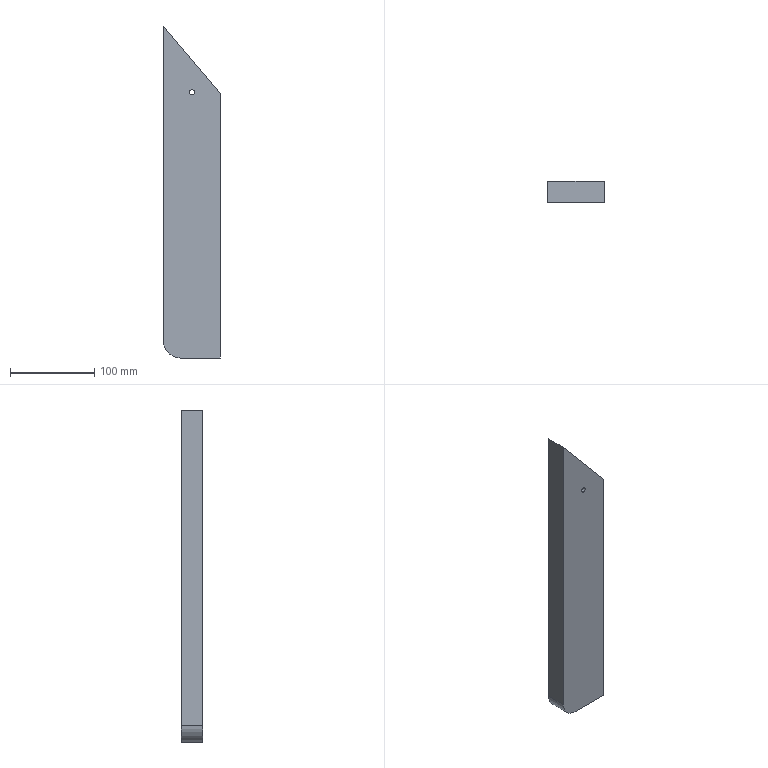Part | SolidWorks | features Extrusion 1, Fillet 1 | 1 solid | 9 faces | box 67.5 x 25 x 394.016 mm | volume 594550 mm3 | plane 6 | cylinder 3 | commonest cylinder face diameters 6 x2 40 x1
STEP:
#1=CARTESIAN_POINT('',(33.75,25.,312.249));
#2=VERTEX_POINT('',#1);
#3=CARTESIAN_POINT('',(33.75,25.,318.249));
#4=VERTEX_POINT('',#3);
#5=CARTESIAN_POINT('',(33.75,25.,315.249));
#6=DIRECTION('',(0.,1.,0.));
#7=DIRECTION('',(0.,0.,1.));
#8=AXIS2_PLACEMENT_3D('',#5,#6,#7);
#9=CIRCLE('',#8,3.);
#10=EDGE_CURVE('',#2,#4,#9,.T.);
#11=ORIENTED_EDGE('',*,*,#10,.T.);
#12=CARTESIAN_POINT('',(33.75,0.,318.249));
#13=VERTEX_POINT('',#12);
#14=CARTESIAN_POINT('',(33.75,25.,318.249));
#15=DIRECTION('',(0.,-1.,0.));
#16=VECTOR('',#15,1000.);
#17=LINE('',#14,#16);
#18=EDGE_CURVE('',#4,#13,#17,.T.);
#19=ORIENTED_EDGE('',*,*,#18,.T.);
#20=CARTESIAN_POINT('',(33.75,0.,312.249));
#21=VERTEX_POINT('',#20);
#22=CARTESIAN_POINT('',(33.75,0.,315.249));
#23=DIRECTION('',(0.,1.,0.));
#24=DIRECTION('',(0.,0.,1.));
#25=AXIS2_PLACEMENT_3D('',#22,#23,#24);
#26=CIRCLE('',#25,3.);
#27=EDGE_CURVE('',#21,#13,#26,.T.);
#28=ORIENTED_EDGE('',*,*,#27,.F.);
#29=CARTESIAN_POINT('',(33.75,25.,312.249));
#30=DIRECTION('',(0.,-1.,0.));
#31=VECTOR('',#30,1000.);
#32=LINE('',#29,#31);
#33=EDGE_CURVE('',#2,#21,#32,.T.);
#34=ORIENTED_EDGE('',*,*,#33,.F.);
#35=EDGE_LOOP('',(#11,#19,#28,#34));
#36=FACE_OUTER_BOUND('',#35,.T.);
#37=CARTESIAN_POINT('',(33.75,25.,315.249));
#38=DIRECTION('',(0.,-1.,0.));
#39=DIRECTION('',(0.,0.,-1.));
#40=AXIS2_PLACEMENT_3D('',#37,#38,#39);
#41=CYLINDRICAL_SURFACE('',#40,3.);
#42=ADVANCED_FACE('',(#36),#41,.F.);
#43=CARTESIAN_POINT('',(67.5,25.,0.));
#44=VERTEX_POINT('',#43);
#45=CARTESIAN_POINT('',(20.,25.,0.));
#46=VERTEX_POINT('',#45);
#47=CARTESIAN_POINT('',(67.5,25.,0.));
#48=DIRECTION('',(-1.,0.,0.));
#49=VECTOR('',#48,1000.);
#50=LINE('',#47,#49);
#51=EDGE_CURVE('',#44,#46,#50,.T.);
#52=ORIENTED_EDGE('',*,*,#51,.T.);
#53=CARTESIAN_POINT('',(0.,25.,20.));
#54=VERTEX_POINT('',#53);
#55=CARTESIAN_POINT('',(20.,25.,20.));
#56=DIRECTION('',(0.,1.,0.));
#57=DIRECTION('',(0.,0.,-1.));
#58=AXIS2_PLACEMENT_3D('',#55,#56,#57);
#59=CIRCLE('',#58,20.);
#60=EDGE_CURVE('',#46,#54,#59,.T.);
#61=ORIENTED_EDGE('',*,*,#60,.T.);
#62=CARTESIAN_POINT('',(0.,25.,394.016));
#63=VERTEX_POINT('',#62);
#64=CARTESIAN_POINT('',(0.,25.,0.));
#65=DIRECTION('',(0.,0.,1.));
#66=VECTOR('',#65,1000.);
#67=LINE('',#64,#66);
#68=EDGE_CURVE('',#54,#63,#67,.T.);
#69=ORIENTED_EDGE('',*,*,#68,.T.);
#70=CARTESIAN_POINT('',(67.5,25.,314.016));
#71=VERTEX_POINT('',#70);
#72=CARTESIAN_POINT('',(67.5,25.,314.016));
#73=DIRECTION('',(0.6449,0.,-0.7643));
#74=VECTOR('',#73,1000.);
#75=LINE('',#72,#74);
#76=EDGE_CURVE('',#63,#71,#75,.T.);
#77=ORIENTED_EDGE('',*,*,#76,.T.);
#78=CARTESIAN_POINT('',(67.5,25.,0.));
#79=DIRECTION('',(0.,0.,-1.));
#80=VECTOR('',#79,1000.);
#81=LINE('',#78,#80);
#82=EDGE_CURVE('',#71,#44,#81,.T.);
#83=ORIENTED_EDGE('',*,*,#82,.T.);
#84=EDGE_LOOP('',(#52,#61,#69,#77,#83));
#85=FACE_OUTER_BOUND('',#84,.T.);
#86=ORIENTED_EDGE('',*,*,#10,.F.);
#87=CARTESIAN_POINT('',(33.75,25.,315.249));
#88=DIRECTION('',(0.,1.,0.));
#89=DIRECTION('',(0.,0.,1.));
#90=AXIS2_PLACEMENT_3D('',#87,#88,#89);
#91=CIRCLE('',#90,3.);
#92=EDGE_CURVE('',#4,#2,#91,.T.);
#93=ORIENTED_EDGE('',*,*,#92,.F.);
#94=EDGE_LOOP('',(#86,#93));
#95=FACE_BOUND('',#94,.T.);
#96=CARTESIAN_POINT('',(0.,25.,0.));
#97=DIRECTION('',(0.,-1.,0.));
#98=DIRECTION('',(0.,0.,-1.));
#99=AXIS2_PLACEMENT_3D('',#96,#97,#98);
#100=PLANE('',#99);
#101=ADVANCED_FACE('',(#85,#95),#100,.F.);
#102=CARTESIAN_POINT('',(0.,0.,20.));
#103=VERTEX_POINT('',#102);
#104=CARTESIAN_POINT('',(0.,0.,394.016));
#105=VERTEX_POINT('',#104);
#106=CARTESIAN_POINT('',(0.,0.,0.));
#107=DIRECTION('',(0.,0.,1.));
#108=VECTOR('',#107,1000.);
#109=LINE('',#106,#108);
#110=EDGE_CURVE('',#103,#105,#109,.T.);
#111=ORIENTED_EDGE('',*,*,#110,.F.);
#112=CARTESIAN_POINT('',(20.,0.,0.));
#113=VERTEX_POINT('',#112);
#114=CARTESIAN_POINT('',(20.,0.,20.));
#115=DIRECTION('',(0.,-1.,0.));
#116=DIRECTION('',(0.,0.,-1.));
#117=AXIS2_PLACEMENT_3D('',#114,#115,#116);
#118=CIRCLE('',#117,20.);
#119=EDGE_CURVE('',#103,#113,#118,.T.);
#120=ORIENTED_EDGE('',*,*,#119,.T.);
#121=CARTESIAN_POINT('',(67.5,0.,0.));
#122=VERTEX_POINT('',#121);
#123=CARTESIAN_POINT('',(67.5,0.,0.));
#124=DIRECTION('',(-1.,0.,0.));
#125=VECTOR('',#124,1000.);
#126=LINE('',#123,#125);
#127=EDGE_CURVE('',#122,#113,#126,.T.);
#128=ORIENTED_EDGE('',*,*,#127,.F.);
#129=CARTESIAN_POINT('',(67.5,0.,314.016));
#130=VERTEX_POINT('',#129);
#131=CARTESIAN_POINT('',(67.5,0.,0.));
#132=DIRECTION('',(0.,0.,-1.));
#133=VECTOR('',#132,1000.);
#134=LINE('',#131,#133);
#135=EDGE_CURVE('',#130,#122,#134,.T.);
#136=ORIENTED_EDGE('',*,*,#135,.F.);
#137=CARTESIAN_POINT('',(67.5,0.,314.016));
#138=DIRECTION('',(0.6449,0.,-0.7643));
#139=VECTOR('',#138,1000.);
#140=LINE('',#137,#139);
#141=EDGE_CURVE('',#105,#130,#140,.T.);
#142=ORIENTED_EDGE('',*,*,#141,.F.);
#143=EDGE_LOOP('',(#111,#120,#128,#136,#142));
#144=FACE_OUTER_BOUND('',#143,.T.);
#145=ORIENTED_EDGE('',*,*,#27,.T.);
#146=CARTESIAN_POINT('',(33.75,0.,315.249));
#147=DIRECTION('',(0.,1.,0.));
#148=DIRECTION('',(0.,0.,1.));
#149=AXIS2_PLACEMENT_3D('',#146,#147,#148);
#150=CIRCLE('',#149,3.);
#151=EDGE_CURVE('',#13,#21,#150,.T.);
#152=ORIENTED_EDGE('',*,*,#151,.T.);
#153=EDGE_LOOP('',(#145,#152));
#154=FACE_BOUND('',#153,.T.);
#155=CARTESIAN_POINT('',(0.,0.,0.));
#156=DIRECTION('',(0.,-1.,0.));
#157=DIRECTION('',(0.,0.,-1.));
#158=AXIS2_PLACEMENT_3D('',#155,#156,#157);
#159=PLANE('',#158);
#160=ADVANCED_FACE('',(#144,#154),#159,.T.);
#161=ORIENTED_EDGE('',*,*,#135,.T.);
#162=CARTESIAN_POINT('',(67.5,25.,0.));
#163=DIRECTION('',(0.,-1.,0.));
#164=VECTOR('',#163,1000.);
#165=LINE('',#162,#164);
#166=EDGE_CURVE('',#44,#122,#165,.T.);
#167=ORIENTED_EDGE('',*,*,#166,.F.);
#168=ORIENTED_EDGE('',*,*,#82,.F.);
#169=CARTESIAN_POINT('',(67.5,25.,314.016));
#170=DIRECTION('',(0.,-1.,0.));
#171=VECTOR('',#170,1000.);
#172=LINE('',#169,#171);
#173=EDGE_CURVE('',#71,#130,#172,.T.);
#174=ORIENTED_EDGE('',*,*,#173,.T.);
#175=EDGE_LOOP('',(#161,#167,#168,#174));
#176=FACE_OUTER_BOUND('',#175,.T.);
#177=CARTESIAN_POINT('',(67.5,25.,0.));
#178=DIRECTION('',(-1.,0.,0.));
#179=DIRECTION('',(0.,0.,1.));
#180=AXIS2_PLACEMENT_3D('',#177,#178,#179);
#181=PLANE('',#180);
#182=ADVANCED_FACE('',(#176),#181,.F.);
#183=ORIENTED_EDGE('',*,*,#127,.T.);
#184=CARTESIAN_POINT('',(20.,25.,0.));
#185=DIRECTION('',(0.,1.,0.));
#186=VECTOR('',#185,1000.);
#187=LINE('',#184,#186);
#188=EDGE_CURVE('',#113,#46,#187,.T.);
#189=ORIENTED_EDGE('',*,*,#188,.T.);
#190=ORIENTED_EDGE('',*,*,#51,.F.);
#191=ORIENTED_EDGE('',*,*,#166,.T.);
#192=EDGE_LOOP('',(#183,#189,#190,#191));
#193=FACE_OUTER_BOUND('',#192,.T.);
#194=CARTESIAN_POINT('',(67.5,25.,0.));
#195=DIRECTION('',(0.,0.,1.));
#196=DIRECTION('',(1.,0.,0.));
#197=AXIS2_PLACEMENT_3D('',#194,#195,#196);
#198=PLANE('',#197);
#199=ADVANCED_FACE('',(#193),#198,.F.);
#200=ORIENTED_EDGE('',*,*,#68,.F.);
#201=CARTESIAN_POINT('',(0.,25.,20.));
#202=DIRECTION('',(0.,-1.,0.));
#203=VECTOR('',#202,1000.);
#204=LINE('',#201,#203);
#205=EDGE_CURVE('',#54,#103,#204,.T.);
#206=ORIENTED_EDGE('',*,*,#205,.T.);
#207=ORIENTED_EDGE('',*,*,#110,.T.);
#208=CARTESIAN_POINT('',(0.,25.,394.016));
#209=DIRECTION('',(0.,-1.,0.));
#210=VECTOR('',#209,1000.);
#211=LINE('',#208,#210);
#212=EDGE_CURVE('',#63,#105,#211,.T.);
#213=ORIENTED_EDGE('',*,*,#212,.F.);
#214=EDGE_LOOP('',(#200,#206,#207,#213));
#215=FACE_OUTER_BOUND('',#214,.T.);
#216=CARTESIAN_POINT('',(0.,25.,0.));
#217=DIRECTION('',(1.,0.,0.));
#218=DIRECTION('',(0.,0.,-1.));
#219=AXIS2_PLACEMENT_3D('',#216,#217,#218);
#220=PLANE('',#219);
#221=ADVANCED_FACE('',(#215),#220,.F.);
#222=ORIENTED_EDGE('',*,*,#141,.T.);
#223=ORIENTED_EDGE('',*,*,#173,.F.);
#224=ORIENTED_EDGE('',*,*,#76,.F.);
#225=ORIENTED_EDGE('',*,*,#212,.T.);
#226=EDGE_LOOP('',(#222,#223,#224,#225));
#227=FACE_OUTER_BOUND('',#226,.T.);
#228=CARTESIAN_POINT('',(67.5,25.,314.016));
#229=DIRECTION('',(-0.7643,0.,-0.6449));
#230=DIRECTION('',(-0.6449,0.,0.7643));
#231=AXIS2_PLACEMENT_3D('',#228,#229,#230);
#232=PLANE('',#231);
#233=ADVANCED_FACE('',(#227),#232,.F.);
#234=ORIENTED_EDGE('',*,*,#18,.F.);
#235=ORIENTED_EDGE('',*,*,#92,.T.);
#236=ORIENTED_EDGE('',*,*,#33,.T.);
#237=ORIENTED_EDGE('',*,*,#151,.F.);
#238=EDGE_LOOP('',(#234,#235,#236,#237));
#239=FACE_OUTER_BOUND('',#238,.T.);
#240=CARTESIAN_POINT('',(33.75,25.,315.249));
#241=DIRECTION('',(0.,-1.,0.));
#242=DIRECTION('',(0.,0.,-1.));
#243=AXIS2_PLACEMENT_3D('',#240,#241,#242);
#244=CYLINDRICAL_SURFACE('',#243,3.);
#245=ADVANCED_FACE('',(#239),#244,.F.);
#246=ORIENTED_EDGE('',*,*,#60,.F.);
#247=ORIENTED_EDGE('',*,*,#188,.F.);
#248=ORIENTED_EDGE('',*,*,#119,.F.);
#249=ORIENTED_EDGE('',*,*,#205,.F.);
#250=EDGE_LOOP('',(#246,#247,#248,#249));
#251=FACE_OUTER_BOUND('',#250,.T.);
#252=CARTESIAN_POINT('',(20.,25.,20.));
#253=DIRECTION('',(0.,-1.,0.));
#254=DIRECTION('',(0.,0.,-1.));
#255=AXIS2_PLACEMENT_3D('',#252,#253,#254);
#256=CYLINDRICAL_SURFACE('',#255,20.);
#257=ADVANCED_FACE('',(#251),#256,.T.);
#258=CLOSED_SHELL('',(#42,#101,#160,#182,#199,#221,#233,#245,#257));
#259=MANIFOLD_SOLID_BREP('',#258);
#260=CARTESIAN_POINT('',(0.,0.,0.));
#261=DIRECTION('',(0.,0.,1.));
#262=DIRECTION('',(1.,0.,0.));
#263=AXIS2_PLACEMENT_3D('',#260,#261,#262);
#264=(LENGTH_UNIT()NAMED_UNIT(*)SI_UNIT(.MILLI.,.METRE.));
#265=UNCERTAINTY_MEASURE_WITH_UNIT(LENGTH_MEASURE(0.00001),#264,'','');
#266=(NAMED_UNIT(*)PLANE_ANGLE_UNIT()SI_UNIT($,.RADIAN.));
#267=(NAMED_UNIT(*)SI_UNIT($,.STERADIAN.)SOLID_ANGLE_UNIT());
#268=(GEOMETRIC_REPRESENTATION_CONTEXT(3)GLOBAL_UNCERTAINTY_ASSIGNED_CONTEXT((#265))GLOBAL_UNIT_ASSIGNED_CONTEXT((#264,#266,#267))REPRESENTATION_CONTEXT('',''));
#269=ADVANCED_BREP_SHAPE_REPRESENTATION('',(#259,#263),#268);